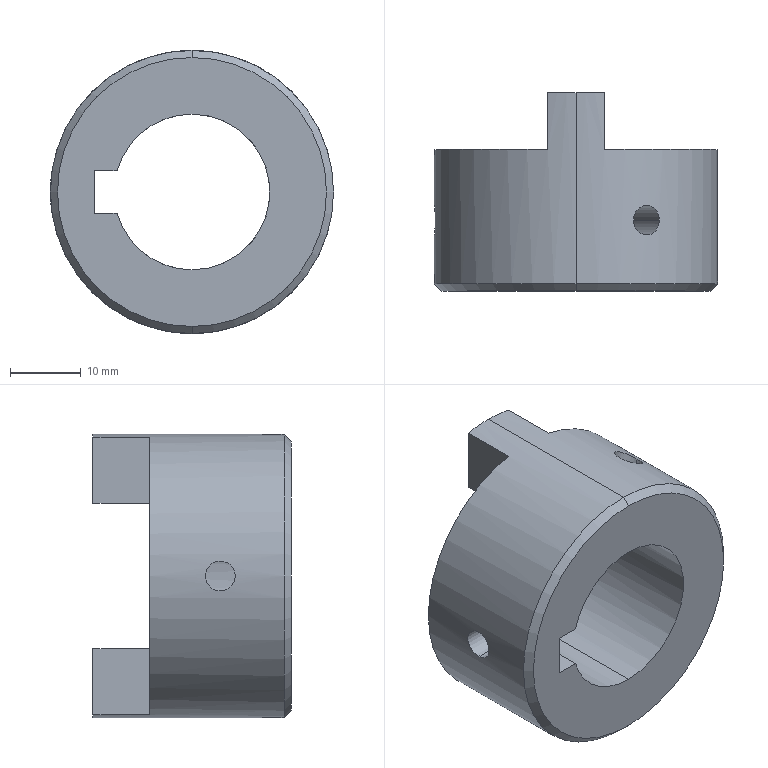Part | STEP file | CON-007 | 1 solid | 23 faces | box 40 x 28 x 40 mm | volume 18074 mm3 | plane 12 | cylinder 9 | cone 2 | commonest cylinder face diameters 4.2 x4 22 x3 40 x2